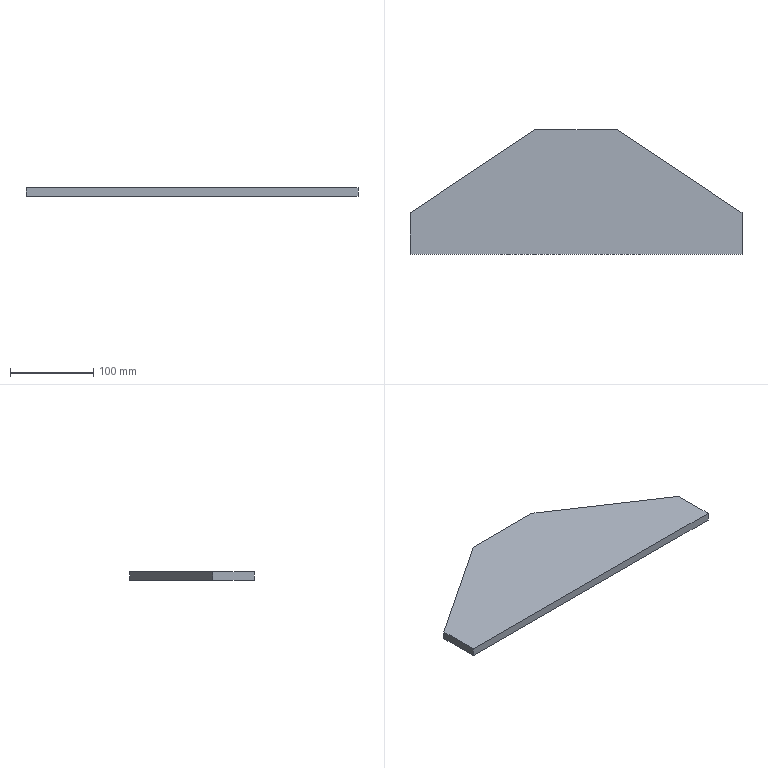Part | SolidWorks | features BaseBody 1 | 1 solid | 8 faces | box 400 x 150 x 10 mm | volume 450000 mm3 | plane 8
STEP:
#1=CARTESIAN_POINT('',(50.,2119.544,-20.));
#2=VERTEX_POINT('',#1);
#3=CARTESIAN_POINT('',(-50.,2119.544,-20.));
#4=VERTEX_POINT('',#3);
#5=CARTESIAN_POINT('',(-240.,2119.544,-20.));
#6=DIRECTION('',(-1.,0.,0.));
#7=VECTOR('',#6,1000.);
#8=LINE('',#5,#7);
#9=EDGE_CURVE('',#2,#4,#8,.T.);
#10=ORIENTED_EDGE('',*,*,#9,.F.);
#11=CARTESIAN_POINT('',(200.,2019.544,-20.));
#12=VERTEX_POINT('',#11);
#13=CARTESIAN_POINT('',(200.,2019.544,-20.));
#14=DIRECTION('',(-0.8321,0.5547,0.));
#15=VECTOR('',#14,1000.);
#16=LINE('',#13,#15);
#17=EDGE_CURVE('',#12,#2,#16,.T.);
#18=ORIENTED_EDGE('',*,*,#17,.F.);
#19=CARTESIAN_POINT('',(200.,1969.544,-20.));
#20=VERTEX_POINT('',#19);
#21=CARTESIAN_POINT('',(200.,2339.544,-20.));
#22=DIRECTION('',(0.,1.,0.));
#23=VECTOR('',#22,1000.);
#24=LINE('',#21,#23);
#25=EDGE_CURVE('',#20,#12,#24,.T.);
#26=ORIENTED_EDGE('',*,*,#25,.F.);
#27=CARTESIAN_POINT('',(-200.,1969.544,-20.));
#28=VERTEX_POINT('',#27);
#29=CARTESIAN_POINT('',(-240.,1969.544,-20.));
#30=DIRECTION('',(1.,0.,0.));
#31=VECTOR('',#30,1000.);
#32=LINE('',#29,#31);
#33=EDGE_CURVE('',#28,#20,#32,.T.);
#34=ORIENTED_EDGE('',*,*,#33,.F.);
#35=CARTESIAN_POINT('',(-200.,2019.544,-20.));
#36=VERTEX_POINT('',#35);
#37=CARTESIAN_POINT('',(-200.,2339.544,-20.));
#38=DIRECTION('',(0.,-1.,0.));
#39=VECTOR('',#38,1000.);
#40=LINE('',#37,#39);
#41=EDGE_CURVE('',#36,#28,#40,.T.);
#42=ORIENTED_EDGE('',*,*,#41,.F.);
#43=CARTESIAN_POINT('',(-50.,2119.544,-20.));
#44=DIRECTION('',(-0.8321,-0.5547,0.));
#45=VECTOR('',#44,1000.);
#46=LINE('',#43,#45);
#47=EDGE_CURVE('',#4,#36,#46,.T.);
#48=ORIENTED_EDGE('',*,*,#47,.F.);
#49=EDGE_LOOP('',(#10,#18,#26,#34,#42,#48));
#50=FACE_OUTER_BOUND('',#49,.T.);
#51=CARTESIAN_POINT('',(-240.,2339.544,-20.));
#52=DIRECTION('',(0.,0.,1.));
#53=DIRECTION('',(1.,0.,0.));
#54=AXIS2_PLACEMENT_3D('',#51,#52,#53);
#55=PLANE('',#54);
#56=ADVANCED_FACE('',(#50),#55,.F.);
#57=CARTESIAN_POINT('',(-50.,2119.544,-10.));
#58=VERTEX_POINT('',#57);
#59=CARTESIAN_POINT('',(-200.,2019.544,-10.));
#60=VERTEX_POINT('',#59);
#61=CARTESIAN_POINT('',(-50.,2119.544,-10.));
#62=DIRECTION('',(-0.8321,-0.5547,0.));
#63=VECTOR('',#62,1000.);
#64=LINE('',#61,#63);
#65=EDGE_CURVE('',#58,#60,#64,.T.);
#66=ORIENTED_EDGE('',*,*,#65,.F.);
#67=CARTESIAN_POINT('',(-50.,2119.544,-10.));
#68=DIRECTION('',(0.,0.,1.));
#69=VECTOR('',#68,1000.);
#70=LINE('',#67,#69);
#71=EDGE_CURVE('',#4,#58,#70,.T.);
#72=ORIENTED_EDGE('',*,*,#71,.F.);
#73=ORIENTED_EDGE('',*,*,#47,.T.);
#74=CARTESIAN_POINT('',(-200.,2019.544,-10.));
#75=DIRECTION('',(0.,0.,-1.));
#76=VECTOR('',#75,1000.);
#77=LINE('',#74,#76);
#78=EDGE_CURVE('',#60,#36,#77,.T.);
#79=ORIENTED_EDGE('',*,*,#78,.F.);
#80=EDGE_LOOP('',(#66,#72,#73,#79));
#81=FACE_OUTER_BOUND('',#80,.T.);
#82=CARTESIAN_POINT('',(-50.,2119.544,-10.));
#83=DIRECTION('',(0.5547,-0.8321,0.));
#84=DIRECTION('',(0.8321,0.5547,0.));
#85=AXIS2_PLACEMENT_3D('',#82,#83,#84);
#86=PLANE('',#85);
#87=ADVANCED_FACE('',(#81),#86,.F.);
#88=CARTESIAN_POINT('',(50.,2119.544,-10.));
#89=VERTEX_POINT('',#88);
#90=CARTESIAN_POINT('',(-50.,2119.544,-10.));
#91=DIRECTION('',(-1.,0.,0.));
#92=VECTOR('',#91,1000.);
#93=LINE('',#90,#92);
#94=EDGE_CURVE('',#89,#58,#93,.T.);
#95=ORIENTED_EDGE('',*,*,#94,.F.);
#96=CARTESIAN_POINT('',(50.,2119.544,-10.));
#97=DIRECTION('',(0.,0.,1.));
#98=VECTOR('',#97,1000.);
#99=LINE('',#96,#98);
#100=EDGE_CURVE('',#2,#89,#99,.T.);
#101=ORIENTED_EDGE('',*,*,#100,.F.);
#102=ORIENTED_EDGE('',*,*,#9,.T.);
#103=ORIENTED_EDGE('',*,*,#71,.T.);
#104=EDGE_LOOP('',(#95,#101,#102,#103));
#105=FACE_OUTER_BOUND('',#104,.T.);
#106=CARTESIAN_POINT('',(-50.,2119.544,-10.));
#107=DIRECTION('',(0.,-1.,0.));
#108=DIRECTION('',(0.,0.,-1.));
#109=AXIS2_PLACEMENT_3D('',#106,#107,#108);
#110=PLANE('',#109);
#111=ADVANCED_FACE('',(#105),#110,.F.);
#112=CARTESIAN_POINT('',(200.,2019.544,-10.));
#113=VERTEX_POINT('',#112);
#114=CARTESIAN_POINT('',(200.,2019.544,-10.));
#115=DIRECTION('',(-0.8321,0.5547,0.));
#116=VECTOR('',#115,1000.);
#117=LINE('',#114,#116);
#118=EDGE_CURVE('',#113,#89,#117,.T.);
#119=ORIENTED_EDGE('',*,*,#118,.F.);
#120=CARTESIAN_POINT('',(200.,2019.544,-10.));
#121=DIRECTION('',(0.,0.,1.));
#122=VECTOR('',#121,1000.);
#123=LINE('',#120,#122);
#124=EDGE_CURVE('',#12,#113,#123,.T.);
#125=ORIENTED_EDGE('',*,*,#124,.F.);
#126=ORIENTED_EDGE('',*,*,#17,.T.);
#127=ORIENTED_EDGE('',*,*,#100,.T.);
#128=EDGE_LOOP('',(#119,#125,#126,#127));
#129=FACE_OUTER_BOUND('',#128,.T.);
#130=CARTESIAN_POINT('',(200.,2019.544,-10.));
#131=DIRECTION('',(-0.5547,-0.8321,0.));
#132=DIRECTION('',(0.8321,-0.5547,0.));
#133=AXIS2_PLACEMENT_3D('',#130,#131,#132);
#134=PLANE('',#133);
#135=ADVANCED_FACE('',(#129),#134,.F.);
#136=CARTESIAN_POINT('',(200.,1969.544,-10.));
#137=VERTEX_POINT('',#136);
#138=CARTESIAN_POINT('',(200.,1969.544,-10.));
#139=DIRECTION('',(0.,1.,0.));
#140=VECTOR('',#139,1000.);
#141=LINE('',#138,#140);
#142=EDGE_CURVE('',#137,#113,#141,.T.);
#143=ORIENTED_EDGE('',*,*,#142,.F.);
#144=CARTESIAN_POINT('',(200.,1969.544,-10.));
#145=DIRECTION('',(0.,0.,1.));
#146=VECTOR('',#145,1000.);
#147=LINE('',#144,#146);
#148=EDGE_CURVE('',#20,#137,#147,.T.);
#149=ORIENTED_EDGE('',*,*,#148,.F.);
#150=ORIENTED_EDGE('',*,*,#25,.T.);
#151=ORIENTED_EDGE('',*,*,#124,.T.);
#152=EDGE_LOOP('',(#143,#149,#150,#151));
#153=FACE_OUTER_BOUND('',#152,.T.);
#154=CARTESIAN_POINT('',(200.,1969.544,-10.));
#155=DIRECTION('',(-1.,0.,0.));
#156=DIRECTION('',(0.,0.,1.));
#157=AXIS2_PLACEMENT_3D('',#154,#155,#156);
#158=PLANE('',#157);
#159=ADVANCED_FACE('',(#153),#158,.F.);
#160=CARTESIAN_POINT('',(-200.,1969.544,-10.));
#161=VERTEX_POINT('',#160);
#162=CARTESIAN_POINT('',(-200.,1969.544,-10.));
#163=DIRECTION('',(1.,0.,0.));
#164=VECTOR('',#163,1000.);
#165=LINE('',#162,#164);
#166=EDGE_CURVE('',#161,#137,#165,.T.);
#167=ORIENTED_EDGE('',*,*,#166,.F.);
#168=CARTESIAN_POINT('',(-200.,1969.544,-10.));
#169=DIRECTION('',(0.,0.,1.));
#170=VECTOR('',#169,1000.);
#171=LINE('',#168,#170);
#172=EDGE_CURVE('',#28,#161,#171,.T.);
#173=ORIENTED_EDGE('',*,*,#172,.F.);
#174=ORIENTED_EDGE('',*,*,#33,.T.);
#175=ORIENTED_EDGE('',*,*,#148,.T.);
#176=EDGE_LOOP('',(#167,#173,#174,#175));
#177=FACE_OUTER_BOUND('',#176,.T.);
#178=CARTESIAN_POINT('',(-200.,1969.544,-10.));
#179=DIRECTION('',(0.,1.,0.));
#180=DIRECTION('',(0.,0.,1.));
#181=AXIS2_PLACEMENT_3D('',#178,#179,#180);
#182=PLANE('',#181);
#183=ADVANCED_FACE('',(#177),#182,.F.);
#184=CARTESIAN_POINT('',(-200.,2019.544,-10.));
#185=DIRECTION('',(0.,-1.,0.));
#186=VECTOR('',#185,1000.);
#187=LINE('',#184,#186);
#188=EDGE_CURVE('',#60,#161,#187,.T.);
#189=ORIENTED_EDGE('',*,*,#188,.F.);
#190=ORIENTED_EDGE('',*,*,#78,.T.);
#191=ORIENTED_EDGE('',*,*,#41,.T.);
#192=ORIENTED_EDGE('',*,*,#172,.T.);
#193=EDGE_LOOP('',(#189,#190,#191,#192));
#194=FACE_OUTER_BOUND('',#193,.T.);
#195=CARTESIAN_POINT('',(-200.,2019.544,-10.));
#196=DIRECTION('',(1.,0.,0.));
#197=DIRECTION('',(0.,0.,-1.));
#198=AXIS2_PLACEMENT_3D('',#195,#196,#197);
#199=PLANE('',#198);
#200=ADVANCED_FACE('',(#194),#199,.F.);
#201=ORIENTED_EDGE('',*,*,#65,.T.);
#202=ORIENTED_EDGE('',*,*,#188,.T.);
#203=ORIENTED_EDGE('',*,*,#166,.T.);
#204=ORIENTED_EDGE('',*,*,#142,.T.);
#205=ORIENTED_EDGE('',*,*,#118,.T.);
#206=ORIENTED_EDGE('',*,*,#94,.T.);
#207=EDGE_LOOP('',(#201,#202,#203,#204,#205,#206));
#208=FACE_OUTER_BOUND('',#207,.T.);
#209=CARTESIAN_POINT('',(-240.,2339.544,-10.));
#210=DIRECTION('',(0.,0.,1.));
#211=DIRECTION('',(1.,0.,0.));
#212=AXIS2_PLACEMENT_3D('',#209,#210,#211);
#213=PLANE('',#212);
#214=ADVANCED_FACE('',(#208),#213,.T.);
#215=CLOSED_SHELL('',(#56,#87,#111,#135,#159,#183,#200,#214));
#216=MANIFOLD_SOLID_BREP('',#215);
#217=CARTESIAN_POINT('',(0.,0.,0.));
#218=DIRECTION('',(0.,0.,1.));
#219=DIRECTION('',(1.,0.,0.));
#220=AXIS2_PLACEMENT_3D('',#217,#218,#219);
#221=(LENGTH_UNIT()NAMED_UNIT(*)SI_UNIT(.MILLI.,.METRE.));
#222=UNCERTAINTY_MEASURE_WITH_UNIT(LENGTH_MEASURE(0.00001),#221,'','');
#223=(NAMED_UNIT(*)PLANE_ANGLE_UNIT()SI_UNIT($,.RADIAN.));
#224=(NAMED_UNIT(*)SI_UNIT($,.STERADIAN.)SOLID_ANGLE_UNIT());
#225=(GEOMETRIC_REPRESENTATION_CONTEXT(3)GLOBAL_UNCERTAINTY_ASSIGNED_CONTEXT((#222))GLOBAL_UNIT_ASSIGNED_CONTEXT((#221,#223,#224))REPRESENTATION_CONTEXT('',''));
#226=ADVANCED_BREP_SHAPE_REPRESENTATION('',(#216,#220),#225);